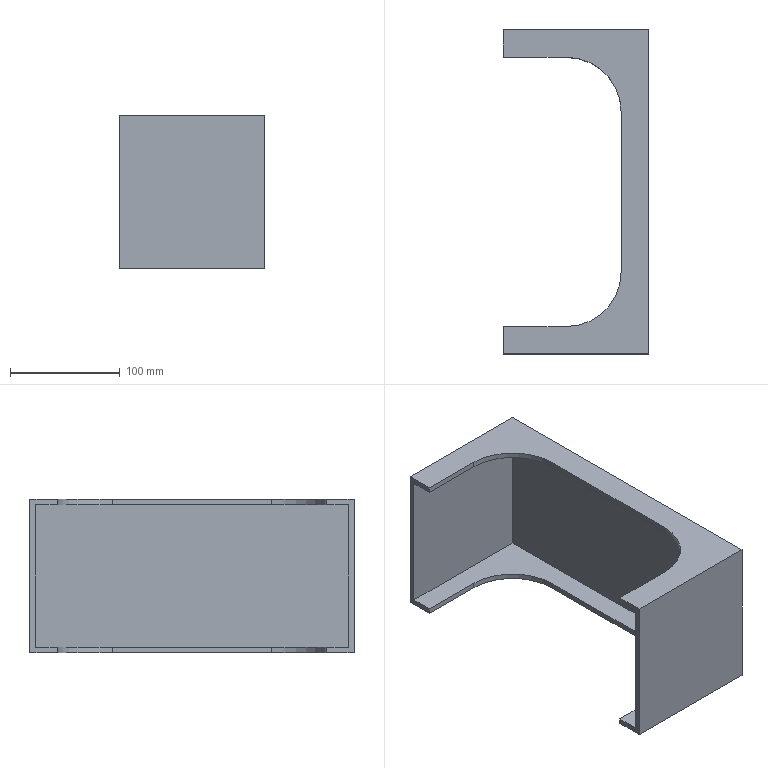Part | NX | features BREP 1 | 1 solid | 22 faces | box 132.305 x 295.254 x 140 mm | volume 495609 mm3 | plane 18 | cylinder 4 | commonest cylinder face diameters 100 x4
STEP:
#1=CARTESIAN_POINT('',(232.792,809.775,135.));
#2=VERTEX_POINT('',#1);
#3=CARTESIAN_POINT('',(232.792,809.775,5.));
#4=VERTEX_POINT('',#3);
#5=CARTESIAN_POINT('',(232.792,809.775,140.));
#6=DIRECTION('',(0.,0.,-1.));
#7=VECTOR('',#6,1000.);
#8=LINE('',#5,#7);
#9=EDGE_CURVE('',#2,#4,#8,.T.);
#10=ORIENTED_EDGE('',*,*,#9,.F.);
#11=CARTESIAN_POINT('',(105.487,809.775,135.));
#12=VERTEX_POINT('',#11);
#13=CARTESIAN_POINT('',(237.792,809.775,135.));
#14=DIRECTION('',(-1.,0.,0.));
#15=VECTOR('',#14,1000.);
#16=LINE('',#13,#15);
#17=EDGE_CURVE('',#2,#12,#16,.T.);
#18=ORIENTED_EDGE('',*,*,#17,.T.);
#19=CARTESIAN_POINT('',(105.487,809.775,5.));
#20=VERTEX_POINT('',#19);
#21=CARTESIAN_POINT('',(105.487,809.775,140.));
#22=DIRECTION('',(0.,0.,1.));
#23=VECTOR('',#22,1000.);
#24=LINE('',#21,#23);
#25=EDGE_CURVE('',#20,#12,#24,.T.);
#26=ORIENTED_EDGE('',*,*,#25,.F.);
#27=CARTESIAN_POINT('',(237.792,809.775,5.));
#28=DIRECTION('',(1.,0.,0.));
#29=VECTOR('',#28,1000.);
#30=LINE('',#27,#29);
#31=EDGE_CURVE('',#20,#4,#30,.T.);
#32=ORIENTED_EDGE('',*,*,#31,.T.);
#33=EDGE_LOOP('',(#10,#18,#26,#32));
#34=FACE_BOUND('',#33,.T.);
#35=CARTESIAN_POINT('',(237.792,809.775,140.));
#36=DIRECTION('',(0.,-1.,0.));
#37=DIRECTION('',(-1.,0.,0.));
#38=AXIS2_PLACEMENT_3D('',#35,#36,#37);
#39=PLANE('',#38);
#40=ADVANCED_FACE('',(#34),#39,.T.);
#41=CARTESIAN_POINT('',(232.792,524.52,135.));
#42=VERTEX_POINT('',#41);
#43=CARTESIAN_POINT('',(232.792,524.52,5.));
#44=VERTEX_POINT('',#43);
#45=CARTESIAN_POINT('',(232.792,524.52,140.));
#46=DIRECTION('',(0.,0.,-1.));
#47=VECTOR('',#46,1000.);
#48=LINE('',#45,#47);
#49=EDGE_CURVE('',#42,#44,#48,.T.);
#50=ORIENTED_EDGE('',*,*,#49,.F.);
#51=CARTESIAN_POINT('',(232.792,519.52,135.));
#52=DIRECTION('',(0.,1.,0.));
#53=VECTOR('',#52,1000.);
#54=LINE('',#51,#53);
#55=EDGE_CURVE('',#42,#2,#54,.T.);
#56=ORIENTED_EDGE('',*,*,#55,.T.);
#57=ORIENTED_EDGE('',*,*,#9,.T.);
#58=CARTESIAN_POINT('',(232.792,519.52,5.));
#59=DIRECTION('',(0.,-1.,0.));
#60=VECTOR('',#59,1000.);
#61=LINE('',#58,#60);
#62=EDGE_CURVE('',#4,#44,#61,.T.);
#63=ORIENTED_EDGE('',*,*,#62,.T.);
#64=EDGE_LOOP('',(#50,#56,#57,#63));
#65=FACE_BOUND('',#64,.T.);
#66=CARTESIAN_POINT('',(232.792,519.52,140.));
#67=DIRECTION('',(-1.,0.,0.));
#68=DIRECTION('',(0.,1.,0.));
#69=AXIS2_PLACEMENT_3D('',#66,#67,#68);
#70=PLANE('',#69);
#71=ADVANCED_FACE('',(#65),#70,.T.);
#72=CARTESIAN_POINT('',(105.487,524.52,135.));
#73=VERTEX_POINT('',#72);
#74=CARTESIAN_POINT('',(105.487,524.52,5.));
#75=VERTEX_POINT('',#74);
#76=CARTESIAN_POINT('',(105.487,524.52,140.));
#77=DIRECTION('',(0.,0.,-1.));
#78=VECTOR('',#77,1000.);
#79=LINE('',#76,#78);
#80=EDGE_CURVE('',#73,#75,#79,.T.);
#81=ORIENTED_EDGE('',*,*,#80,.F.);
#82=CARTESIAN_POINT('',(105.487,524.52,135.));
#83=DIRECTION('',(1.,0.,0.));
#84=VECTOR('',#83,1000.);
#85=LINE('',#82,#84);
#86=EDGE_CURVE('',#73,#42,#85,.T.);
#87=ORIENTED_EDGE('',*,*,#86,.T.);
#88=ORIENTED_EDGE('',*,*,#49,.T.);
#89=CARTESIAN_POINT('',(105.487,524.52,5.));
#90=DIRECTION('',(-1.,0.,0.));
#91=VECTOR('',#90,1000.);
#92=LINE('',#89,#91);
#93=EDGE_CURVE('',#44,#75,#92,.T.);
#94=ORIENTED_EDGE('',*,*,#93,.T.);
#95=EDGE_LOOP('',(#81,#87,#88,#94));
#96=FACE_BOUND('',#95,.T.);
#97=CARTESIAN_POINT('',(105.487,524.52,140.));
#98=DIRECTION('',(0.,1.,0.));
#99=DIRECTION('',(1.,0.,0.));
#100=AXIS2_PLACEMENT_3D('',#97,#98,#99);
#101=PLANE('',#100);
#102=ADVANCED_FACE('',(#96),#101,.T.);
#103=CARTESIAN_POINT('',(105.487,544.52,0.));
#104=VERTEX_POINT('',#103);
#105=CARTESIAN_POINT('',(105.487,519.52,0.));
#106=VERTEX_POINT('',#105);
#107=CARTESIAN_POINT('',(105.487,519.52,0.));
#108=DIRECTION('',(0.,-1.,0.));
#109=VECTOR('',#108,1000.);
#110=LINE('',#107,#109);
#111=EDGE_CURVE('',#104,#106,#110,.T.);
#112=ORIENTED_EDGE('',*,*,#111,.T.);
#113=CARTESIAN_POINT('',(105.487,519.52,140.));
#114=VERTEX_POINT('',#113);
#115=CARTESIAN_POINT('',(105.487,519.52,140.));
#116=DIRECTION('',(0.,0.,-1.));
#117=VECTOR('',#116,1000.);
#118=LINE('',#115,#117);
#119=EDGE_CURVE('',#114,#106,#118,.T.);
#120=ORIENTED_EDGE('',*,*,#119,.F.);
#121=CARTESIAN_POINT('',(105.487,544.52,140.));
#122=VERTEX_POINT('',#121);
#123=CARTESIAN_POINT('',(105.487,519.52,140.));
#124=DIRECTION('',(0.,-1.,0.));
#125=VECTOR('',#124,1000.);
#126=LINE('',#123,#125);
#127=EDGE_CURVE('',#122,#114,#126,.T.);
#128=ORIENTED_EDGE('',*,*,#127,.F.);
#129=CARTESIAN_POINT('',(105.487,544.52,135.));
#130=VERTEX_POINT('',#129);
#131=CARTESIAN_POINT('',(105.487,544.52,135.));
#132=DIRECTION('',(0.,0.,1.));
#133=VECTOR('',#132,1000.);
#134=LINE('',#131,#133);
#135=EDGE_CURVE('',#130,#122,#134,.T.);
#136=ORIENTED_EDGE('',*,*,#135,.F.);
#137=CARTESIAN_POINT('',(105.487,519.52,135.));
#138=DIRECTION('',(0.,1.,0.));
#139=VECTOR('',#138,1000.);
#140=LINE('',#137,#139);
#141=EDGE_CURVE('',#73,#130,#140,.T.);
#142=ORIENTED_EDGE('',*,*,#141,.F.);
#143=ORIENTED_EDGE('',*,*,#80,.T.);
#144=CARTESIAN_POINT('',(105.487,544.52,5.));
#145=VERTEX_POINT('',#144);
#146=CARTESIAN_POINT('',(105.487,544.52,5.));
#147=DIRECTION('',(0.,1.,0.));
#148=VECTOR('',#147,1000.);
#149=LINE('',#146,#148);
#150=EDGE_CURVE('',#75,#145,#149,.T.);
#151=ORIENTED_EDGE('',*,*,#150,.T.);
#152=CARTESIAN_POINT('',(105.487,544.52,0.));
#153=DIRECTION('',(0.,0.,1.));
#154=VECTOR('',#153,1000.);
#155=LINE('',#152,#154);
#156=EDGE_CURVE('',#104,#145,#155,.T.);
#157=ORIENTED_EDGE('',*,*,#156,.F.);
#158=EDGE_LOOP('',(#112,#120,#128,#136,#142,#143,#151,#157));
#159=FACE_BOUND('',#158,.T.);
#160=CARTESIAN_POINT('',(105.487,519.52,140.));
#161=DIRECTION('',(1.,0.,0.));
#162=DIRECTION('',(0.,0.,1.));
#163=AXIS2_PLACEMENT_3D('',#160,#161,#162);
#164=PLANE('',#163);
#165=ADVANCED_FACE('',(#159),#164,.F.);
#166=CARTESIAN_POINT('',(162.792,544.52,140.));
#167=VERTEX_POINT('',#166);
#168=CARTESIAN_POINT('',(105.487,544.52,140.));
#169=DIRECTION('',(1.,0.,0.));
#170=VECTOR('',#169,1000.);
#171=LINE('',#168,#170);
#172=EDGE_CURVE('',#122,#167,#171,.T.);
#173=ORIENTED_EDGE('',*,*,#172,.F.);
#174=ORIENTED_EDGE('',*,*,#127,.T.);
#175=CARTESIAN_POINT('',(237.792,519.52,140.));
#176=VERTEX_POINT('',#175);
#177=CARTESIAN_POINT('',(105.487,519.52,140.));
#178=DIRECTION('',(-1.,0.,0.));
#179=VECTOR('',#178,1000.);
#180=LINE('',#177,#179);
#181=EDGE_CURVE('',#176,#114,#180,.T.);
#182=ORIENTED_EDGE('',*,*,#181,.F.);
#183=CARTESIAN_POINT('',(237.792,814.775,140.));
#184=VERTEX_POINT('',#183);
#185=CARTESIAN_POINT('',(237.792,519.52,140.));
#186=DIRECTION('',(0.,-1.,0.));
#187=VECTOR('',#186,1000.);
#188=LINE('',#185,#187);
#189=EDGE_CURVE('',#184,#176,#188,.T.);
#190=ORIENTED_EDGE('',*,*,#189,.F.);
#191=CARTESIAN_POINT('',(105.487,814.775,140.));
#192=VERTEX_POINT('',#191);
#193=CARTESIAN_POINT('',(237.792,814.775,140.));
#194=DIRECTION('',(1.,0.,0.));
#195=VECTOR('',#194,1000.);
#196=LINE('',#193,#195);
#197=EDGE_CURVE('',#192,#184,#196,.T.);
#198=ORIENTED_EDGE('',*,*,#197,.F.);
#199=CARTESIAN_POINT('',(105.487,789.775,140.));
#200=VERTEX_POINT('',#199);
#201=CARTESIAN_POINT('',(105.487,814.775,140.));
#202=DIRECTION('',(0.,1.,0.));
#203=VECTOR('',#202,1000.);
#204=LINE('',#201,#203);
#205=EDGE_CURVE('',#200,#192,#204,.T.);
#206=ORIENTED_EDGE('',*,*,#205,.F.);
#207=CARTESIAN_POINT('',(162.792,789.775,140.));
#208=VERTEX_POINT('',#207);
#209=CARTESIAN_POINT('',(162.792,789.775,140.));
#210=DIRECTION('',(-1.,0.,0.));
#211=VECTOR('',#210,1000.);
#212=LINE('',#209,#211);
#213=EDGE_CURVE('',#208,#200,#212,.T.);
#214=ORIENTED_EDGE('',*,*,#213,.F.);
#215=CARTESIAN_POINT('',(212.792,739.775,140.));
#216=VERTEX_POINT('',#215);
#217=CARTESIAN_POINT('',(162.792,739.775,140.));
#218=DIRECTION('',(0.,0.,1.));
#219=DIRECTION('',(1.,0.,0.));
#220=AXIS2_PLACEMENT_3D('',#217,#218,#219);
#221=CIRCLE('',#220,50.);
#222=EDGE_CURVE('',#216,#208,#221,.T.);
#223=ORIENTED_EDGE('',*,*,#222,.F.);
#224=CARTESIAN_POINT('',(212.792,594.52,140.));
#225=VERTEX_POINT('',#224);
#226=CARTESIAN_POINT('',(212.792,594.52,140.));
#227=DIRECTION('',(0.,1.,0.));
#228=VECTOR('',#227,1000.);
#229=LINE('',#226,#228);
#230=EDGE_CURVE('',#225,#216,#229,.T.);
#231=ORIENTED_EDGE('',*,*,#230,.F.);
#232=CARTESIAN_POINT('',(162.792,594.52,140.));
#233=DIRECTION('',(0.,0.,1.));
#234=DIRECTION('',(1.,0.,0.));
#235=AXIS2_PLACEMENT_3D('',#232,#233,#234);
#236=CIRCLE('',#235,50.);
#237=EDGE_CURVE('',#167,#225,#236,.T.);
#238=ORIENTED_EDGE('',*,*,#237,.F.);
#239=EDGE_LOOP('',(#173,#174,#182,#190,#198,#206,#214,#223,#231,#238));
#240=FACE_BOUND('',#239,.T.);
#241=CARTESIAN_POINT('',(237.792,814.775,140.));
#242=DIRECTION('',(0.,0.,1.));
#243=DIRECTION('',(1.,0.,0.));
#244=AXIS2_PLACEMENT_3D('',#241,#242,#243);
#245=PLANE('',#244);
#246=ADVANCED_FACE('',(#240),#245,.T.);
#247=ORIENTED_EDGE('',*,*,#25,.T.);
#248=CARTESIAN_POINT('',(105.487,789.775,135.));
#249=VERTEX_POINT('',#248);
#250=CARTESIAN_POINT('',(105.487,789.775,135.));
#251=DIRECTION('',(0.,1.,0.));
#252=VECTOR('',#251,1000.);
#253=LINE('',#250,#252);
#254=EDGE_CURVE('',#249,#12,#253,.T.);
#255=ORIENTED_EDGE('',*,*,#254,.F.);
#256=CARTESIAN_POINT('',(105.487,789.775,135.));
#257=DIRECTION('',(0.,0.,1.));
#258=VECTOR('',#257,1000.);
#259=LINE('',#256,#258);
#260=EDGE_CURVE('',#249,#200,#259,.T.);
#261=ORIENTED_EDGE('',*,*,#260,.T.);
#262=ORIENTED_EDGE('',*,*,#205,.T.);
#263=CARTESIAN_POINT('',(105.487,814.775,0.));
#264=VERTEX_POINT('',#263);
#265=CARTESIAN_POINT('',(105.487,814.775,140.));
#266=DIRECTION('',(0.,0.,1.));
#267=VECTOR('',#266,1000.);
#268=LINE('',#265,#267);
#269=EDGE_CURVE('',#264,#192,#268,.T.);
#270=ORIENTED_EDGE('',*,*,#269,.F.);
#271=CARTESIAN_POINT('',(105.487,789.775,0.));
#272=VERTEX_POINT('',#271);
#273=CARTESIAN_POINT('',(105.487,814.775,0.));
#274=DIRECTION('',(0.,1.,0.));
#275=VECTOR('',#274,1000.);
#276=LINE('',#273,#275);
#277=EDGE_CURVE('',#272,#264,#276,.T.);
#278=ORIENTED_EDGE('',*,*,#277,.F.);
#279=CARTESIAN_POINT('',(105.487,789.775,5.));
#280=VERTEX_POINT('',#279);
#281=CARTESIAN_POINT('',(105.487,789.775,0.));
#282=DIRECTION('',(0.,0.,1.));
#283=VECTOR('',#282,1000.);
#284=LINE('',#281,#283);
#285=EDGE_CURVE('',#272,#280,#284,.T.);
#286=ORIENTED_EDGE('',*,*,#285,.T.);
#287=CARTESIAN_POINT('',(105.487,814.775,5.));
#288=DIRECTION('',(0.,1.,0.));
#289=VECTOR('',#288,1000.);
#290=LINE('',#287,#289);
#291=EDGE_CURVE('',#280,#20,#290,.T.);
#292=ORIENTED_EDGE('',*,*,#291,.T.);
#293=EDGE_LOOP('',(#247,#255,#261,#262,#270,#278,#286,#292));
#294=FACE_BOUND('',#293,.T.);
#295=CARTESIAN_POINT('',(105.487,814.775,140.));
#296=DIRECTION('',(-1.,0.,0.));
#297=DIRECTION('',(0.,0.,1.));
#298=AXIS2_PLACEMENT_3D('',#295,#296,#297);
#299=PLANE('',#298);
#300=ADVANCED_FACE('',(#294),#299,.T.);
#301=CARTESIAN_POINT('',(162.792,789.775,0.));
#302=VERTEX_POINT('',#301);
#303=CARTESIAN_POINT('',(105.487,789.775,0.));
#304=DIRECTION('',(1.,0.,0.));
#305=VECTOR('',#304,1000.);
#306=LINE('',#303,#305);
#307=EDGE_CURVE('',#272,#302,#306,.T.);
#308=ORIENTED_EDGE('',*,*,#307,.F.);
#309=ORIENTED_EDGE('',*,*,#277,.T.);
#310=CARTESIAN_POINT('',(237.792,814.775,0.));
#311=VERTEX_POINT('',#310);
#312=CARTESIAN_POINT('',(237.792,814.775,0.));
#313=DIRECTION('',(-1.,0.,0.));
#314=VECTOR('',#313,1000.);
#315=LINE('',#312,#314);
#316=EDGE_CURVE('',#311,#264,#315,.T.);
#317=ORIENTED_EDGE('',*,*,#316,.F.);
#318=CARTESIAN_POINT('',(237.792,519.52,0.));
#319=VERTEX_POINT('',#318);
#320=CARTESIAN_POINT('',(237.792,519.52,0.));
#321=DIRECTION('',(0.,1.,0.));
#322=VECTOR('',#321,1000.);
#323=LINE('',#320,#322);
#324=EDGE_CURVE('',#319,#311,#323,.T.);
#325=ORIENTED_EDGE('',*,*,#324,.F.);
#326=CARTESIAN_POINT('',(105.487,519.52,0.));
#327=DIRECTION('',(1.,0.,0.));
#328=VECTOR('',#327,1000.);
#329=LINE('',#326,#328);
#330=EDGE_CURVE('',#106,#319,#329,.T.);
#331=ORIENTED_EDGE('',*,*,#330,.F.);
#332=ORIENTED_EDGE('',*,*,#111,.F.);
#333=CARTESIAN_POINT('',(162.792,544.52,0.));
#334=VERTEX_POINT('',#333);
#335=CARTESIAN_POINT('',(162.792,544.52,0.));
#336=DIRECTION('',(-1.,0.,0.));
#337=VECTOR('',#336,1000.);
#338=LINE('',#335,#337);
#339=EDGE_CURVE('',#334,#104,#338,.T.);
#340=ORIENTED_EDGE('',*,*,#339,.F.);
#341=CARTESIAN_POINT('',(212.792,594.52,0.));
#342=VERTEX_POINT('',#341);
#343=CARTESIAN_POINT('',(162.792,594.52,0.));
#344=DIRECTION('',(0.,0.,-1.));
#345=DIRECTION('',(1.,0.,0.));
#346=AXIS2_PLACEMENT_3D('',#343,#344,#345);
#347=CIRCLE('',#346,50.);
#348=EDGE_CURVE('',#342,#334,#347,.T.);
#349=ORIENTED_EDGE('',*,*,#348,.F.);
#350=CARTESIAN_POINT('',(212.792,739.775,0.));
#351=VERTEX_POINT('',#350);
#352=CARTESIAN_POINT('',(212.792,739.775,0.));
#353=DIRECTION('',(0.,-1.,0.));
#354=VECTOR('',#353,1000.);
#355=LINE('',#352,#354);
#356=EDGE_CURVE('',#351,#342,#355,.T.);
#357=ORIENTED_EDGE('',*,*,#356,.F.);
#358=CARTESIAN_POINT('',(162.792,739.775,0.));
#359=DIRECTION('',(0.,0.,-1.));
#360=DIRECTION('',(1.,0.,0.));
#361=AXIS2_PLACEMENT_3D('',#358,#359,#360);
#362=CIRCLE('',#361,50.);
#363=EDGE_CURVE('',#302,#351,#362,.T.);
#364=ORIENTED_EDGE('',*,*,#363,.F.);
#365=EDGE_LOOP('',(#308,#309,#317,#325,#331,#332,#340,#349,#357,#364));
#366=FACE_BOUND('',#365,.T.);
#367=CARTESIAN_POINT('',(237.792,519.52,0.));
#368=DIRECTION('',(0.,0.,1.));
#369=DIRECTION('',(0.,-1.,0.));
#370=AXIS2_PLACEMENT_3D('',#367,#368,#369);
#371=PLANE('',#370);
#372=ADVANCED_FACE('',(#366),#371,.F.);
#373=ORIENTED_EDGE('',*,*,#269,.T.);
#374=ORIENTED_EDGE('',*,*,#197,.T.);
#375=CARTESIAN_POINT('',(237.792,814.775,140.));
#376=DIRECTION('',(0.,0.,-1.));
#377=VECTOR('',#376,1000.);
#378=LINE('',#375,#377);
#379=EDGE_CURVE('',#184,#311,#378,.T.);
#380=ORIENTED_EDGE('',*,*,#379,.T.);
#381=ORIENTED_EDGE('',*,*,#316,.T.);
#382=EDGE_LOOP('',(#373,#374,#380,#381));
#383=FACE_BOUND('',#382,.T.);
#384=CARTESIAN_POINT('',(237.792,814.775,140.));
#385=DIRECTION('',(0.,-1.,0.));
#386=DIRECTION('',(-1.,0.,0.));
#387=AXIS2_PLACEMENT_3D('',#384,#385,#386);
#388=PLANE('',#387);
#389=ADVANCED_FACE('',(#383),#388,.F.);
#390=ORIENTED_EDGE('',*,*,#324,.T.);
#391=ORIENTED_EDGE('',*,*,#379,.F.);
#392=ORIENTED_EDGE('',*,*,#189,.T.);
#393=CARTESIAN_POINT('',(237.792,519.52,140.));
#394=DIRECTION('',(0.,0.,-1.));
#395=VECTOR('',#394,1000.);
#396=LINE('',#393,#395);
#397=EDGE_CURVE('',#176,#319,#396,.T.);
#398=ORIENTED_EDGE('',*,*,#397,.T.);
#399=EDGE_LOOP('',(#390,#391,#392,#398));
#400=FACE_BOUND('',#399,.T.);
#401=CARTESIAN_POINT('',(237.792,519.52,140.));
#402=DIRECTION('',(-1.,0.,0.));
#403=DIRECTION('',(0.,1.,0.));
#404=AXIS2_PLACEMENT_3D('',#401,#402,#403);
#405=PLANE('',#404);
#406=ADVANCED_FACE('',(#400),#405,.F.);
#407=ORIENTED_EDGE('',*,*,#330,.T.);
#408=ORIENTED_EDGE('',*,*,#397,.F.);
#409=ORIENTED_EDGE('',*,*,#181,.T.);
#410=ORIENTED_EDGE('',*,*,#119,.T.);
#411=EDGE_LOOP('',(#407,#408,#409,#410));
#412=FACE_BOUND('',#411,.T.);
#413=CARTESIAN_POINT('',(105.487,519.52,140.));
#414=DIRECTION('',(0.,1.,0.));
#415=DIRECTION('',(1.,0.,0.));
#416=AXIS2_PLACEMENT_3D('',#413,#414,#415);
#417=PLANE('',#416);
#418=ADVANCED_FACE('',(#412),#417,.F.);
#419=CARTESIAN_POINT('',(162.792,789.775,5.));
#420=VERTEX_POINT('',#419);
#421=CARTESIAN_POINT('',(105.487,789.775,5.));
#422=DIRECTION('',(1.,0.,0.));
#423=VECTOR('',#422,1000.);
#424=LINE('',#421,#423);
#425=EDGE_CURVE('',#280,#420,#424,.T.);
#426=ORIENTED_EDGE('',*,*,#425,.F.);
#427=ORIENTED_EDGE('',*,*,#285,.F.);
#428=ORIENTED_EDGE('',*,*,#307,.T.);
#429=CARTESIAN_POINT('',(162.792,789.775,0.));
#430=DIRECTION('',(0.,0.,1.));
#431=VECTOR('',#430,1000.);
#432=LINE('',#429,#431);
#433=EDGE_CURVE('',#302,#420,#432,.T.);
#434=ORIENTED_EDGE('',*,*,#433,.T.);
#435=EDGE_LOOP('',(#426,#427,#428,#434));
#436=FACE_BOUND('',#435,.T.);
#437=CARTESIAN_POINT('',(105.487,789.775,0.));
#438=DIRECTION('',(0.,-1.,0.));
#439=DIRECTION('',(-1.,0.,0.));
#440=AXIS2_PLACEMENT_3D('',#437,#438,#439);
#441=PLANE('',#440);
#442=ADVANCED_FACE('',(#436),#441,.T.);
#443=CARTESIAN_POINT('',(212.792,739.775,5.));
#444=VERTEX_POINT('',#443);
#445=CARTESIAN_POINT('',(162.792,739.775,5.));
#446=DIRECTION('',(0.,0.,-1.));
#447=DIRECTION('',(1.,0.,0.));
#448=AXIS2_PLACEMENT_3D('',#445,#446,#447);
#449=CIRCLE('',#448,50.);
#450=EDGE_CURVE('',#420,#444,#449,.T.);
#451=ORIENTED_EDGE('',*,*,#450,.F.);
#452=ORIENTED_EDGE('',*,*,#433,.F.);
#453=ORIENTED_EDGE('',*,*,#363,.T.);
#454=CARTESIAN_POINT('',(212.792,739.775,0.));
#455=DIRECTION('',(0.,0.,1.));
#456=VECTOR('',#455,1000.);
#457=LINE('',#454,#456);
#458=EDGE_CURVE('',#351,#444,#457,.T.);
#459=ORIENTED_EDGE('',*,*,#458,.T.);
#460=EDGE_LOOP('',(#451,#452,#453,#459));
#461=FACE_BOUND('',#460,.T.);
#462=CARTESIAN_POINT('',(162.792,739.775,0.));
#463=DIRECTION('',(0.,0.,1.));
#464=DIRECTION('',(-1.,0.,0.));
#465=AXIS2_PLACEMENT_3D('',#462,#463,#464);
#466=CYLINDRICAL_SURFACE('',#465,50.);
#467=ADVANCED_FACE('',(#461),#466,.F.);
#468=CARTESIAN_POINT('',(212.792,594.52,5.));
#469=VERTEX_POINT('',#468);
#470=CARTESIAN_POINT('',(212.792,739.775,5.));
#471=DIRECTION('',(0.,-1.,0.));
#472=VECTOR('',#471,1000.);
#473=LINE('',#470,#472);
#474=EDGE_CURVE('',#444,#469,#473,.T.);
#475=ORIENTED_EDGE('',*,*,#474,.F.);
#476=ORIENTED_EDGE('',*,*,#458,.F.);
#477=ORIENTED_EDGE('',*,*,#356,.T.);
#478=CARTESIAN_POINT('',(212.792,594.52,0.));
#479=DIRECTION('',(0.,0.,1.));
#480=VECTOR('',#479,1000.);
#481=LINE('',#478,#480);
#482=EDGE_CURVE('',#342,#469,#481,.T.);
#483=ORIENTED_EDGE('',*,*,#482,.T.);
#484=EDGE_LOOP('',(#475,#476,#477,#483));
#485=FACE_BOUND('',#484,.T.);
#486=CARTESIAN_POINT('',(212.792,739.775,0.));
#487=DIRECTION('',(-1.,0.,0.));
#488=DIRECTION('',(0.,1.,0.));
#489=AXIS2_PLACEMENT_3D('',#486,#487,#488);
#490=PLANE('',#489);
#491=ADVANCED_FACE('',(#485),#490,.T.);
#492=CARTESIAN_POINT('',(162.792,544.52,5.));
#493=VERTEX_POINT('',#492);
#494=CARTESIAN_POINT('',(162.792,594.52,5.));
#495=DIRECTION('',(0.,0.,-1.));
#496=DIRECTION('',(1.,0.,0.));
#497=AXIS2_PLACEMENT_3D('',#494,#495,#496);
#498=CIRCLE('',#497,50.);
#499=EDGE_CURVE('',#469,#493,#498,.T.);
#500=ORIENTED_EDGE('',*,*,#499,.F.);
#501=ORIENTED_EDGE('',*,*,#482,.F.);
#502=ORIENTED_EDGE('',*,*,#348,.T.);
#503=CARTESIAN_POINT('',(162.792,544.52,0.));
#504=DIRECTION('',(0.,0.,1.));
#505=VECTOR('',#504,1000.);
#506=LINE('',#503,#505);
#507=EDGE_CURVE('',#334,#493,#506,.T.);
#508=ORIENTED_EDGE('',*,*,#507,.T.);
#509=EDGE_LOOP('',(#500,#501,#502,#508));
#510=FACE_BOUND('',#509,.T.);
#511=CARTESIAN_POINT('',(162.792,594.52,0.));
#512=DIRECTION('',(0.,0.,1.));
#513=DIRECTION('',(-1.,0.,0.));
#514=AXIS2_PLACEMENT_3D('',#511,#512,#513);
#515=CYLINDRICAL_SURFACE('',#514,50.);
#516=ADVANCED_FACE('',(#510),#515,.F.);
#517=CARTESIAN_POINT('',(162.792,544.52,5.));
#518=DIRECTION('',(-1.,0.,0.));
#519=VECTOR('',#518,1000.);
#520=LINE('',#517,#519);
#521=EDGE_CURVE('',#493,#145,#520,.T.);
#522=ORIENTED_EDGE('',*,*,#521,.F.);
#523=ORIENTED_EDGE('',*,*,#507,.F.);
#524=ORIENTED_EDGE('',*,*,#339,.T.);
#525=ORIENTED_EDGE('',*,*,#156,.T.);
#526=EDGE_LOOP('',(#522,#523,#524,#525));
#527=FACE_BOUND('',#526,.T.);
#528=CARTESIAN_POINT('',(162.792,544.52,0.));
#529=DIRECTION('',(0.,1.,0.));
#530=DIRECTION('',(1.,0.,0.));
#531=AXIS2_PLACEMENT_3D('',#528,#529,#530);
#532=PLANE('',#531);
#533=ADVANCED_FACE('',(#527),#532,.T.);
#534=ORIENTED_EDGE('',*,*,#31,.F.);
#535=ORIENTED_EDGE('',*,*,#291,.F.);
#536=ORIENTED_EDGE('',*,*,#425,.T.);
#537=ORIENTED_EDGE('',*,*,#450,.T.);
#538=ORIENTED_EDGE('',*,*,#474,.T.);
#539=ORIENTED_EDGE('',*,*,#499,.T.);
#540=ORIENTED_EDGE('',*,*,#521,.T.);
#541=ORIENTED_EDGE('',*,*,#150,.F.);
#542=ORIENTED_EDGE('',*,*,#93,.F.);
#543=ORIENTED_EDGE('',*,*,#62,.F.);
#544=EDGE_LOOP('',(#534,#535,#536,#537,#538,#539,#540,#541,#542,#543));
#545=FACE_BOUND('',#544,.T.);
#546=CARTESIAN_POINT('',(162.792,739.775,5.));
#547=DIRECTION('',(0.,0.,-1.));
#548=DIRECTION('',(1.,0.,0.));
#549=AXIS2_PLACEMENT_3D('',#546,#547,#548);
#550=PLANE('',#549);
#551=ADVANCED_FACE('',(#545),#550,.F.);
#552=ORIENTED_EDGE('',*,*,#172,.T.);
#553=CARTESIAN_POINT('',(162.792,544.52,135.));
#554=VERTEX_POINT('',#553);
#555=CARTESIAN_POINT('',(162.792,544.52,135.));
#556=DIRECTION('',(0.,0.,1.));
#557=VECTOR('',#556,1000.);
#558=LINE('',#555,#557);
#559=EDGE_CURVE('',#554,#167,#558,.T.);
#560=ORIENTED_EDGE('',*,*,#559,.F.);
#561=CARTESIAN_POINT('',(105.487,544.52,135.));
#562=DIRECTION('',(1.,0.,0.));
#563=VECTOR('',#562,1000.);
#564=LINE('',#561,#563);
#565=EDGE_CURVE('',#130,#554,#564,.T.);
#566=ORIENTED_EDGE('',*,*,#565,.F.);
#567=ORIENTED_EDGE('',*,*,#135,.T.);
#568=EDGE_LOOP('',(#552,#560,#566,#567));
#569=FACE_BOUND('',#568,.T.);
#570=CARTESIAN_POINT('',(105.487,544.52,135.));
#571=DIRECTION('',(0.,-1.,0.));
#572=DIRECTION('',(-1.,0.,0.));
#573=AXIS2_PLACEMENT_3D('',#570,#571,#572);
#574=PLANE('',#573);
#575=ADVANCED_FACE('',(#569),#574,.F.);
#576=ORIENTED_EDGE('',*,*,#237,.T.);
#577=CARTESIAN_POINT('',(212.792,594.52,135.));
#578=VERTEX_POINT('',#577);
#579=CARTESIAN_POINT('',(212.792,594.52,135.));
#580=DIRECTION('',(0.,0.,1.));
#581=VECTOR('',#580,1000.);
#582=LINE('',#579,#581);
#583=EDGE_CURVE('',#578,#225,#582,.T.);
#584=ORIENTED_EDGE('',*,*,#583,.F.);
#585=CARTESIAN_POINT('',(162.792,594.52,135.));
#586=DIRECTION('',(0.,0.,1.));
#587=DIRECTION('',(1.,0.,0.));
#588=AXIS2_PLACEMENT_3D('',#585,#586,#587);
#589=CIRCLE('',#588,50.);
#590=EDGE_CURVE('',#554,#578,#589,.T.);
#591=ORIENTED_EDGE('',*,*,#590,.F.);
#592=ORIENTED_EDGE('',*,*,#559,.T.);
#593=EDGE_LOOP('',(#576,#584,#591,#592));
#594=FACE_BOUND('',#593,.T.);
#595=CARTESIAN_POINT('',(162.792,594.52,135.));
#596=DIRECTION('',(0.,0.,1.));
#597=DIRECTION('',(-1.,0.,0.));
#598=AXIS2_PLACEMENT_3D('',#595,#596,#597);
#599=CYLINDRICAL_SURFACE('',#598,50.);
#600=ADVANCED_FACE('',(#594),#599,.F.);
#601=ORIENTED_EDGE('',*,*,#230,.T.);
#602=CARTESIAN_POINT('',(212.792,739.775,135.));
#603=VERTEX_POINT('',#602);
#604=CARTESIAN_POINT('',(212.792,739.775,135.));
#605=DIRECTION('',(0.,0.,1.));
#606=VECTOR('',#605,1000.);
#607=LINE('',#604,#606);
#608=EDGE_CURVE('',#603,#216,#607,.T.);
#609=ORIENTED_EDGE('',*,*,#608,.F.);
#610=CARTESIAN_POINT('',(212.792,594.52,135.));
#611=DIRECTION('',(0.,1.,0.));
#612=VECTOR('',#611,1000.);
#613=LINE('',#610,#612);
#614=EDGE_CURVE('',#578,#603,#613,.T.);
#615=ORIENTED_EDGE('',*,*,#614,.F.);
#616=ORIENTED_EDGE('',*,*,#583,.T.);
#617=EDGE_LOOP('',(#601,#609,#615,#616));
#618=FACE_BOUND('',#617,.T.);
#619=CARTESIAN_POINT('',(212.792,594.52,135.));
#620=DIRECTION('',(1.,0.,0.));
#621=DIRECTION('',(0.,-1.,0.));
#622=AXIS2_PLACEMENT_3D('',#619,#620,#621);
#623=PLANE('',#622);
#624=ADVANCED_FACE('',(#618),#623,.F.);
#625=ORIENTED_EDGE('',*,*,#222,.T.);
#626=CARTESIAN_POINT('',(162.792,789.775,135.));
#627=VERTEX_POINT('',#626);
#628=CARTESIAN_POINT('',(162.792,789.775,135.));
#629=DIRECTION('',(0.,0.,1.));
#630=VECTOR('',#629,1000.);
#631=LINE('',#628,#630);
#632=EDGE_CURVE('',#627,#208,#631,.T.);
#633=ORIENTED_EDGE('',*,*,#632,.F.);
#634=CARTESIAN_POINT('',(162.792,739.775,135.));
#635=DIRECTION('',(0.,0.,1.));
#636=DIRECTION('',(1.,0.,0.));
#637=AXIS2_PLACEMENT_3D('',#634,#635,#636);
#638=CIRCLE('',#637,50.);
#639=EDGE_CURVE('',#603,#627,#638,.T.);
#640=ORIENTED_EDGE('',*,*,#639,.F.);
#641=ORIENTED_EDGE('',*,*,#608,.T.);
#642=EDGE_LOOP('',(#625,#633,#640,#641));
#643=FACE_BOUND('',#642,.T.);
#644=CARTESIAN_POINT('',(162.792,739.775,135.));
#645=DIRECTION('',(0.,0.,1.));
#646=DIRECTION('',(-1.,0.,0.));
#647=AXIS2_PLACEMENT_3D('',#644,#645,#646);
#648=CYLINDRICAL_SURFACE('',#647,50.);
#649=ADVANCED_FACE('',(#643),#648,.F.);
#650=ORIENTED_EDGE('',*,*,#213,.T.);
#651=ORIENTED_EDGE('',*,*,#260,.F.);
#652=CARTESIAN_POINT('',(162.792,789.775,135.));
#653=DIRECTION('',(-1.,0.,0.));
#654=VECTOR('',#653,1000.);
#655=LINE('',#652,#654);
#656=EDGE_CURVE('',#627,#249,#655,.T.);
#657=ORIENTED_EDGE('',*,*,#656,.F.);
#658=ORIENTED_EDGE('',*,*,#632,.T.);
#659=EDGE_LOOP('',(#650,#651,#657,#658));
#660=FACE_BOUND('',#659,.T.);
#661=CARTESIAN_POINT('',(162.792,789.775,135.));
#662=DIRECTION('',(0.,1.,0.));
#663=DIRECTION('',(1.,0.,0.));
#664=AXIS2_PLACEMENT_3D('',#661,#662,#663);
#665=PLANE('',#664);
#666=ADVANCED_FACE('',(#660),#665,.F.);
#667=ORIENTED_EDGE('',*,*,#17,.F.);
#668=ORIENTED_EDGE('',*,*,#55,.F.);
#669=ORIENTED_EDGE('',*,*,#86,.F.);
#670=ORIENTED_EDGE('',*,*,#141,.T.);
#671=ORIENTED_EDGE('',*,*,#565,.T.);
#672=ORIENTED_EDGE('',*,*,#590,.T.);
#673=ORIENTED_EDGE('',*,*,#614,.T.);
#674=ORIENTED_EDGE('',*,*,#639,.T.);
#675=ORIENTED_EDGE('',*,*,#656,.T.);
#676=ORIENTED_EDGE('',*,*,#254,.T.);
#677=EDGE_LOOP('',(#667,#668,#669,#670,#671,#672,#673,#674,#675,#676));
#678=FACE_BOUND('',#677,.T.);
#679=CARTESIAN_POINT('',(162.792,594.52,135.));
#680=DIRECTION('',(0.,0.,1.));
#681=DIRECTION('',(-1.,0.,0.));
#682=AXIS2_PLACEMENT_3D('',#679,#680,#681);
#683=PLANE('',#682);
#684=ADVANCED_FACE('',(#678),#683,.F.);
#685=CLOSED_SHELL('',(#40,#71,#102,#165,#246,#300,#372,#389,#406,#418,#442,#467,#491,#516,#533,#551,#575,#600,#624,#649,#666,#684));
#686=MANIFOLD_SOLID_BREP('',#685);
#687=(LENGTH_UNIT()NAMED_UNIT(*)SI_UNIT(.MILLI.,.METRE.));
#688=UNCERTAINTY_MEASURE_WITH_UNIT(LENGTH_MEASURE(0.00001),#687,'','');
#689=(NAMED_UNIT(*)PLANE_ANGLE_UNIT()SI_UNIT($,.RADIAN.));
#690=(NAMED_UNIT(*)SI_UNIT($,.STERADIAN.)SOLID_ANGLE_UNIT());
#691=(GEOMETRIC_REPRESENTATION_CONTEXT(3)GLOBAL_UNCERTAINTY_ASSIGNED_CONTEXT((#688))GLOBAL_UNIT_ASSIGNED_CONTEXT((#687,#689,#690))REPRESENTATION_CONTEXT('',''));
#692=ADVANCED_BREP_SHAPE_REPRESENTATION('',(#686),#691);